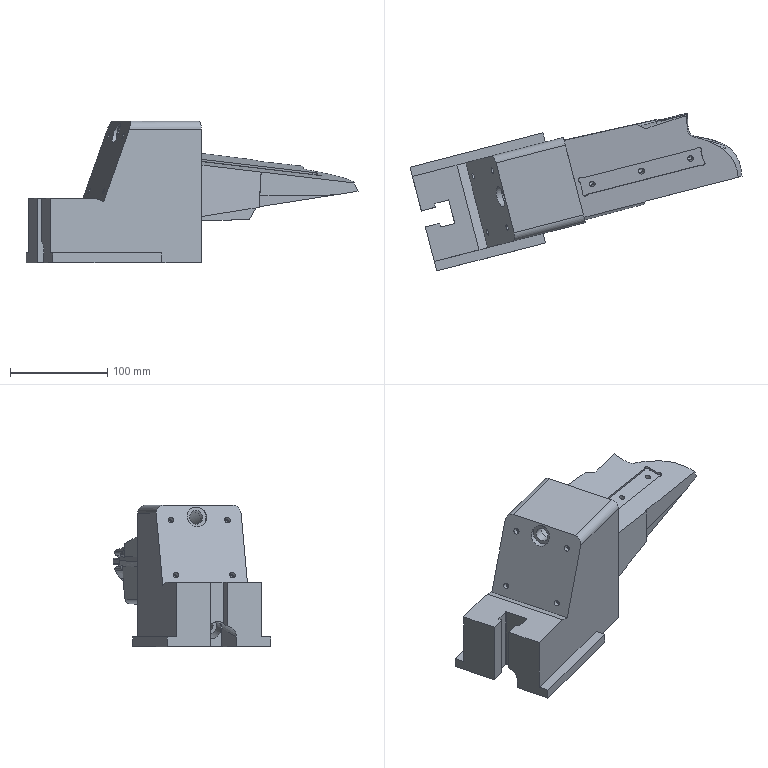Part | STEP file | 车灯-后视镜_id238_x_t | 1 solid | 210 faces | box 340.675 x 161.916 x 145 mm | volume 1865094 mm3 | plane 87 | cylinder 51 | spline 51 | other 10 | cone 10 | sphere 1 | commonest cylinder face diameters 6 x18 5.1 x10 1 x6 21 x4 10 x3 8 x2